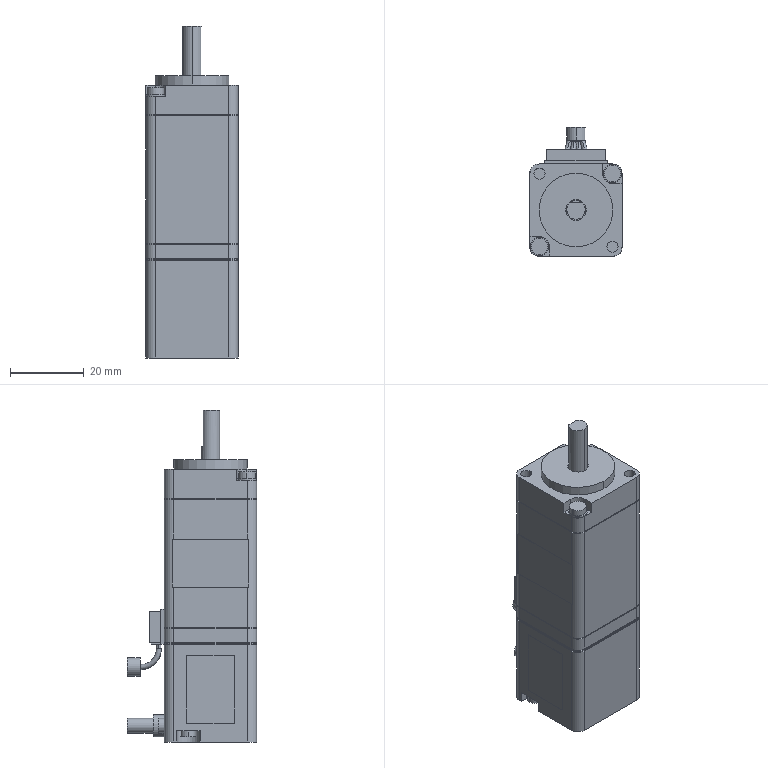Part | SolidWorks | features BaseBody 1, ICE 1 | 1 solid | 206 faces | box 25.2 x 35 x 90 mm | volume 47544 mm3 | plane 109 | cylinder 89 | torus 8 | commonest cylinder face diameters 5 x28 1.36 x16 4.6 x16 4 x10 3 x4 4.5 x4